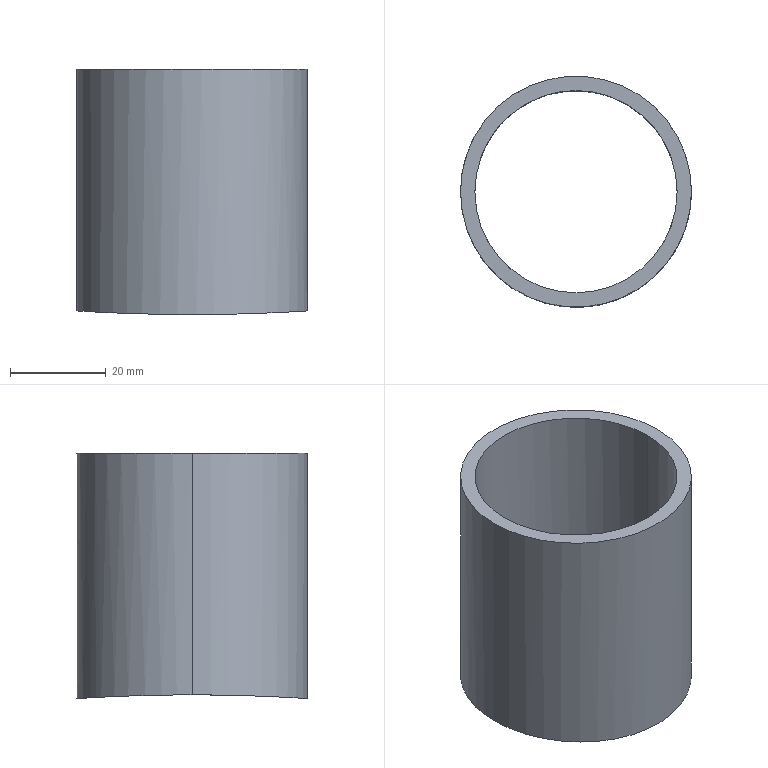Part | SolidWorks | features Extrusion 1, ICE 1 | 1 solid | 6 faces | box 48.3 x 48.3 x 51.269 mm | volume 21706 mm3 | cylinder 5 | plane 1 | commonest cylinder face diameters 42.3 x2 48.3 x2 759 x1
STEP:
#1=CARTESIAN_POINT('',(-21.15,0.,100.));
#2=VERTEX_POINT('',#1);
#3=CARTESIAN_POINT('',(21.15,0.,100.));
#4=VERTEX_POINT('',#3);
#5=CARTESIAN_POINT('',(0.,0.,100.));
#6=DIRECTION('',(0.,0.,1.));
#7=DIRECTION('',(1.,0.,0.));
#8=AXIS2_PLACEMENT_3D('',#5,#6,#7);
#9=CIRCLE('',#8,21.15);
#10=EDGE_CURVE('',#2,#4,#9,.T.);
#11=ORIENTED_EDGE('',*,*,#10,.T.);
#12=CARTESIAN_POINT('',(21.15,0.,49.5));
#13=VERTEX_POINT('',#12);
#14=CARTESIAN_POINT('',(21.15,0.,100.));
#15=DIRECTION('',(0.,0.,-1.));
#16=VECTOR('',#15,1000.);
#17=LINE('',#14,#16);
#18=EDGE_CURVE('',#4,#13,#17,.T.);
#19=ORIENTED_EDGE('',*,*,#18,.T.);
#20=CARTESIAN_POINT('',(-21.15,0.,49.5));
#21=VERTEX_POINT('',#20);
#22=CARTESIAN_POINT('',(-21.15,0.,49.5));
#23=CARTESIAN_POINT('',(-21.15,-1.398,49.5));
#24=CARTESIAN_POINT('',(-21.013,-2.772,49.492));
#25=CARTESIAN_POINT('',(-20.61,-4.8,49.47));
#26=CARTESIAN_POINT('',(-20.442,-5.47,49.461));
#27=CARTESIAN_POINT('',(-20.039,-6.799,49.44));
#28=CARTESIAN_POINT('',(-19.803,-7.46,49.427));
#29=CARTESIAN_POINT('',(-19.007,-9.381,49.386));
#30=CARTESIAN_POINT('',(-18.357,-10.595,49.354));
#31=CARTESIAN_POINT('',(-17.205,-12.32,49.3));
#32=CARTESIAN_POINT('',(-16.79,-12.88,49.282));
#33=CARTESIAN_POINT('',(-15.906,-13.958,49.244));
#34=CARTESIAN_POINT('',(-15.44,-14.47,49.224));
#35=CARTESIAN_POINT('',(-13.977,-15.933,49.167));
#36=CARTESIAN_POINT('',(-12.912,-16.809,49.128));
#37=CARTESIAN_POINT('',(-11.467,-17.775,49.084));
#38=CARTESIAN_POINT('',(-11.171,-17.962,49.075));
#39=CARTESIAN_POINT('',(-10.574,-18.32,49.058));
#40=CARTESIAN_POINT('',(-10.272,-18.491,49.049));
#41=CARTESIAN_POINT('',(-9.356,-18.981,49.025));
#42=CARTESIAN_POINT('',(-8.109,-19.57,48.995));
#43=CARTESIAN_POINT('',(-6.811,-20.035,48.971));
#44=CARTESIAN_POINT('',(-5.818,-20.337,48.955));
#45=CARTESIAN_POINT('',(-5.483,-20.43,48.95));
#46=CARTESIAN_POINT('',(-4.808,-20.599,48.941));
#47=CARTESIAN_POINT('',(-4.467,-20.676,48.936));
#48=CARTESIAN_POINT('',(-2.76,-21.015,48.918));
#49=CARTESIAN_POINT('',(-1.387,-21.15,48.91));
#50=CARTESIAN_POINT('',(0.6823,-21.15,48.91));
#51=CARTESIAN_POINT('',(1.374,-21.117,48.912));
#52=CARTESIAN_POINT('',(2.414,-21.015,48.918));
#53=CARTESIAN_POINT('',(2.762,-20.972,48.92));
#54=CARTESIAN_POINT('',(3.45,-20.87,48.926));
#55=CARTESIAN_POINT('',(3.791,-20.81,48.929));
#56=CARTESIAN_POINT('',(5.487,-20.473,48.947));
#57=CARTESIAN_POINT('',(6.805,-20.073,48.969));
#58=CARTESIAN_POINT('',(8.726,-19.278,49.01));
#59=CARTESIAN_POINT('',(9.36,-18.979,49.025));
#60=CARTESIAN_POINT('',(10.585,-18.324,49.058));
#61=CARTESIAN_POINT('',(11.178,-17.968,49.075));
#62=CARTESIAN_POINT('',(12.896,-16.82,49.128));
#63=CARTESIAN_POINT('',(13.965,-15.946,49.166));
#64=CARTESIAN_POINT('',(15.94,-13.971,49.244));
#65=CARTESIAN_POINT('',(16.816,-12.902,49.282));
#66=CARTESIAN_POINT('',(17.964,-11.184,49.336));
#67=CARTESIAN_POINT('',(18.32,-10.592,49.353));
#68=CARTESIAN_POINT('',(18.975,-9.368,49.385));
#69=CARTESIAN_POINT('',(19.275,-8.734,49.4));
#70=CARTESIAN_POINT('',(20.071,-6.812,49.441));
#71=CARTESIAN_POINT('',(20.471,-5.493,49.463));
#72=CARTESIAN_POINT('',(20.876,-3.46,49.485));
#73=CARTESIAN_POINT('',(20.979,-2.772,49.491));
#74=CARTESIAN_POINT('',(21.116,-1.383,49.498));
#75=CARTESIAN_POINT('',(21.15,-0.6902,49.5));
#76=CARTESIAN_POINT('',(21.15,0.,49.5));
#77=B_SPLINE_CURVE_WITH_KNOTS('',3,(#22,#23,#24,#25,#26,#27,#28,#29,#30,#31,#32,#33,#34,#35,#36,#37,#38,#39,#40,#41,#42,#43,#44,#45,#46,#47,#48,#49,#50,#51,#52,#53,#54,#55,#56,#57,#58,#59,#60,#61,#62,#63,#64,#65,#66,#67,#68,#69,#70,#71,#72,#73,#74,#75,#76),.UNSPECIFIED.,.F.,.F.,(4,2,2,2,2,2,2,2,2,2,1,2,2,2,2,2,2,2,2,2,2,2,2,2,2,2,2,4),(0.,0.004134,0.0062,0.008267,0.0124,0.01447,0.01653,0.02067,0.0217,0.02273,0.0248,0.02687,0.0279,0.02894,0.03307,0.03514,0.03617,0.0372,0.04134,0.0434,0.04547,0.0496,0.05374,0.0558,0.05787,0.062,0.06407,0.06614),.UNSPECIFIED.);
#78=EDGE_CURVE('',#21,#13,#77,.T.);
#79=ORIENTED_EDGE('',*,*,#78,.F.);
#80=CARTESIAN_POINT('',(-21.15,0.,100.));
#81=DIRECTION('',(0.,0.,-1.));
#82=VECTOR('',#81,1000.);
#83=LINE('',#80,#82);
#84=EDGE_CURVE('',#2,#21,#83,.T.);
#85=ORIENTED_EDGE('',*,*,#84,.F.);
#86=EDGE_LOOP('',(#11,#19,#79,#85));
#87=FACE_OUTER_BOUND('',#86,.T.);
#88=CARTESIAN_POINT('',(0.,0.,100.));
#89=DIRECTION('',(0.,0.,-1.));
#90=DIRECTION('',(-1.,0.,0.));
#91=AXIS2_PLACEMENT_3D('',#88,#89,#90);
#92=CYLINDRICAL_SURFACE('',#91,21.15);
#93=ADVANCED_FACE('',(#87),#92,.F.);
#94=CARTESIAN_POINT('',(24.15,0.,100.));
#95=VERTEX_POINT('',#94);
#96=CARTESIAN_POINT('',(-24.15,0.,100.));
#97=VERTEX_POINT('',#96);
#98=CARTESIAN_POINT('',(0.,0.,100.));
#99=DIRECTION('',(0.,0.,1.));
#100=DIRECTION('',(1.,0.,0.));
#101=AXIS2_PLACEMENT_3D('',#98,#99,#100);
#102=CIRCLE('',#101,24.15);
#103=EDGE_CURVE('',#95,#97,#102,.T.);
#104=ORIENTED_EDGE('',*,*,#103,.F.);
#105=CARTESIAN_POINT('',(24.15,0.,49.5));
#106=VERTEX_POINT('',#105);
#107=CARTESIAN_POINT('',(24.15,0.,100.));
#108=DIRECTION('',(0.,0.,-1.));
#109=VECTOR('',#108,1000.);
#110=LINE('',#107,#109);
#111=EDGE_CURVE('',#95,#106,#110,.T.);
#112=ORIENTED_EDGE('',*,*,#111,.T.);
#113=CARTESIAN_POINT('',(-24.15,0.,49.5));
#114=VERTEX_POINT('',#113);
#115=CARTESIAN_POINT('',(24.15,0.,49.5));
#116=CARTESIAN_POINT('',(24.15,1.576,49.5));
#117=CARTESIAN_POINT('',(23.997,3.143,49.49));
#118=CARTESIAN_POINT('',(23.611,5.089,49.466));
#119=CARTESIAN_POINT('',(23.524,5.479,49.461));
#120=CARTESIAN_POINT('',(23.331,6.25,49.449));
#121=CARTESIAN_POINT('',(23.225,6.633,49.442));
#122=CARTESIAN_POINT('',(22.88,7.767,49.421));
#123=CARTESIAN_POINT('',(22.35,9.25,49.389));
#124=CARTESIAN_POINT('',(21.678,10.674,49.351));
#125=CARTESIAN_POINT('',(21.12,11.719,49.319));
#126=CARTESIAN_POINT('',(20.925,12.063,49.308));
#127=CARTESIAN_POINT('',(20.517,12.745,49.286));
#128=CARTESIAN_POINT('',(20.303,13.082,49.275));
#129=CARTESIAN_POINT('',(19.2,14.734,49.216));
#130=CARTESIAN_POINT('',(18.201,15.951,49.166));
#131=CARTESIAN_POINT('',(16.532,17.622,49.091));
#132=CARTESIAN_POINT('',(15.948,18.153,49.066));
#133=CARTESIAN_POINT('',(15.027,18.91,49.029));
#134=CARTESIAN_POINT('',(14.712,19.156,49.016));
#135=CARTESIAN_POINT('',(14.074,19.629,48.992));
#136=CARTESIAN_POINT('',(13.751,19.857,48.98));
#137=CARTESIAN_POINT('',(12.11,20.954,48.922));
#138=CARTESIAN_POINT('',(10.724,21.696,48.88));
#139=CARTESIAN_POINT('',(8.899,22.454,48.835));
#140=CARTESIAN_POINT('',(8.529,22.597,48.827));
#141=CARTESIAN_POINT('',(7.78,22.866,48.811));
#142=CARTESIAN_POINT('',(7.401,22.992,48.803));
#143=CARTESIAN_POINT('',(6.262,23.338,48.782));
#144=CARTESIAN_POINT('',(5.496,23.529,48.77));
#145=CARTESIAN_POINT('',(3.181,23.991,48.741));
#146=CARTESIAN_POINT('',(1.613,24.149,48.731));
#147=CARTESIAN_POINT('',(-0.7771,24.151,48.731));
#148=CARTESIAN_POINT('',(-1.571,24.112,48.733));
#149=CARTESIAN_POINT('',(-3.141,23.958,48.743));
#150=CARTESIAN_POINT('',(-3.92,23.843,48.75));
#151=CARTESIAN_POINT('',(-5.463,23.537,48.769));
#152=CARTESIAN_POINT('',(-6.228,23.347,48.781));
#153=CARTESIAN_POINT('',(-7.744,22.888,48.809));
#154=CARTESIAN_POINT('',(-8.498,22.619,48.825));
#155=CARTESIAN_POINT('',(-10.694,21.711,48.879));
#156=CARTESIAN_POINT('',(-12.082,20.97,48.921));
#157=CARTESIAN_POINT('',(-14.05,19.658,48.991));
#158=CARTESIAN_POINT('',(-14.688,19.186,49.015));
#159=CARTESIAN_POINT('',(-15.921,18.177,49.065));
#160=CARTESIAN_POINT('',(-16.507,17.645,49.09));
#161=CARTESIAN_POINT('',(-18.179,15.975,49.165));
#162=CARTESIAN_POINT('',(-19.179,14.761,49.215));
#163=CARTESIAN_POINT('',(-20.504,12.785,49.285));
#164=CARTESIAN_POINT('',(-20.916,12.099,49.308));
#165=CARTESIAN_POINT('',(-21.662,10.704,49.35));
#166=CARTESIAN_POINT('',(-22.,9.993,49.369));
#167=CARTESIAN_POINT('',(-22.603,8.54,49.405));
#168=CARTESIAN_POINT('',(-22.869,7.8,49.421));
#169=CARTESIAN_POINT('',(-23.33,6.29,49.449));
#170=CARTESIAN_POINT('',(-23.525,5.517,49.461));
#171=CARTESIAN_POINT('',(-23.993,3.174,49.49));
#172=CARTESIAN_POINT('',(-24.15,1.596,49.5));
#173=CARTESIAN_POINT('',(-24.15,0.,49.5));
#174=B_SPLINE_CURVE_WITH_KNOTS('',3,(#115,#116,#117,#118,#119,#120,#121,#122,#123,#124,#125,#126,#127,#128,#129,#130,#131,#132,#133,#134,#135,#136,#137,#138,#139,#140,#141,#142,#143,#144,#145,#146,#147,#148,#149,#150,#151,#152,#153,#154,#155,#156,#157,#158,#159,#160,#161,#162,#163,#164,#165,#166,#167,#168,#169,#170,#171,#172,#173),.UNSPECIFIED.,.F.,.F.,(4,2,2,2,1,2,2,2,2,2,2,2,2,2,2,2,2,2,2,2,2,2,2,2,2,2,2,2,2,4),(0.07552,0.08024,0.08142,0.0826,0.08496,0.08732,0.0885,0.08968,0.0944,0.09676,0.09794,0.09912,0.1038,0.105,0.1062,0.1086,0.1133,0.1156,0.118,0.1204,0.1227,0.1274,0.1298,0.1322,0.1369,0.1392,0.1416,0.144,0.1463,0.151),.UNSPECIFIED.);
#175=EDGE_CURVE('',#106,#114,#174,.T.);
#176=ORIENTED_EDGE('',*,*,#175,.T.);
#177=CARTESIAN_POINT('',(-24.15,0.,100.));
#178=DIRECTION('',(0.,0.,-1.));
#179=VECTOR('',#178,1000.);
#180=LINE('',#177,#179);
#181=EDGE_CURVE('',#97,#114,#180,.T.);
#182=ORIENTED_EDGE('',*,*,#181,.F.);
#183=EDGE_LOOP('',(#104,#112,#176,#182));
#184=FACE_OUTER_BOUND('',#183,.T.);
#185=CARTESIAN_POINT('',(0.,0.,100.));
#186=DIRECTION('',(0.,0.,-1.));
#187=DIRECTION('',(-1.,0.,0.));
#188=AXIS2_PLACEMENT_3D('',#185,#186,#187);
#189=CYLINDRICAL_SURFACE('',#188,24.15);
#190=ADVANCED_FACE('',(#184),#189,.T.);
#191=CARTESIAN_POINT('',(0.,0.,100.));
#192=DIRECTION('',(0.,0.,1.));
#193=DIRECTION('',(1.,0.,0.));
#194=AXIS2_PLACEMENT_3D('',#191,#192,#193);
#195=CIRCLE('',#194,24.15);
#196=EDGE_CURVE('',#97,#95,#195,.T.);
#197=ORIENTED_EDGE('',*,*,#196,.T.);
#198=ORIENTED_EDGE('',*,*,#103,.T.);
#199=EDGE_LOOP('',(#197,#198));
#200=FACE_OUTER_BOUND('',#199,.T.);
#201=ORIENTED_EDGE('',*,*,#10,.F.);
#202=CARTESIAN_POINT('',(0.,0.,100.));
#203=DIRECTION('',(0.,0.,1.));
#204=DIRECTION('',(1.,0.,0.));
#205=AXIS2_PLACEMENT_3D('',#202,#203,#204);
#206=CIRCLE('',#205,21.15);
#207=EDGE_CURVE('',#4,#2,#206,.T.);
#208=ORIENTED_EDGE('',*,*,#207,.F.);
#209=EDGE_LOOP('',(#201,#208));
#210=FACE_BOUND('',#209,.T.);
#211=CARTESIAN_POINT('',(0.,0.,100.));
#212=DIRECTION('',(0.,0.,1.));
#213=DIRECTION('',(1.,0.,0.));
#214=AXIS2_PLACEMENT_3D('',#211,#212,#213);
#215=PLANE('',#214);
#216=ADVANCED_FACE('',(#200,#210),#215,.T.);
#217=ORIENTED_EDGE('',*,*,#111,.F.);
#218=ORIENTED_EDGE('',*,*,#196,.F.);
#219=ORIENTED_EDGE('',*,*,#181,.T.);
#220=CARTESIAN_POINT('',(-24.15,0.,49.5));
#221=CARTESIAN_POINT('',(-24.15,-1.596,49.5));
#222=CARTESIAN_POINT('',(-23.993,-3.165,49.49));
#223=CARTESIAN_POINT('',(-23.533,-5.481,49.461));
#224=CARTESIAN_POINT('',(-23.342,-6.246,49.449));
#225=CARTESIAN_POINT('',(-22.882,-7.764,49.421));
#226=CARTESIAN_POINT('',(-22.612,-8.518,49.405));
#227=CARTESIAN_POINT('',(-21.702,-10.711,49.352));
#228=CARTESIAN_POINT('',(-20.96,-12.099,49.309));
#229=CARTESIAN_POINT('',(-19.865,-13.739,49.251));
#230=CARTESIAN_POINT('',(-19.637,-14.063,49.239));
#231=CARTESIAN_POINT('',(-19.165,-14.7,49.215));
#232=CARTESIAN_POINT('',(-18.919,-15.015,49.203));
#233=CARTESIAN_POINT('',(-18.162,-15.937,49.166));
#234=CARTESIAN_POINT('',(-17.63,-16.523,49.141));
#235=CARTESIAN_POINT('',(-15.959,-18.193,49.065));
#236=CARTESIAN_POINT('',(-14.744,-19.193,49.015));
#237=CARTESIAN_POINT('',(-13.094,-20.296,48.957));
#238=CARTESIAN_POINT('',(-12.756,-20.51,48.945));
#239=CARTESIAN_POINT('',(-12.074,-20.919,48.923));
#240=CARTESIAN_POINT('',(-11.729,-21.114,48.912));
#241=CARTESIAN_POINT('',(-10.684,-21.673,48.881));
#242=CARTESIAN_POINT('',(-9.26,-22.346,48.842));
#243=CARTESIAN_POINT('',(-7.777,-22.877,48.81));
#244=CARTESIAN_POINT('',(-6.643,-23.222,48.789));
#245=CARTESIAN_POINT('',(-6.261,-23.328,48.782));
#246=CARTESIAN_POINT('',(-5.49,-23.521,48.77));
#247=CARTESIAN_POINT('',(-5.1,-23.609,48.765));
#248=CARTESIAN_POINT('',(-3.152,-23.996,48.741));
#249=CARTESIAN_POINT('',(-1.584,-24.149,48.731));
#250=CARTESIAN_POINT('',(0.7792,-24.15,48.731));
#251=CARTESIAN_POINT('',(1.569,-24.112,48.733));
#252=CARTESIAN_POINT('',(2.757,-23.995,48.741));
#253=CARTESIAN_POINT('',(3.154,-23.946,48.744));
#254=CARTESIAN_POINT('',(3.939,-23.83,48.751));
#255=CARTESIAN_POINT('',(4.329,-23.762,48.755));
#256=CARTESIAN_POINT('',(6.265,-23.377,48.779));
#257=CARTESIAN_POINT('',(7.771,-22.92,48.808));
#258=CARTESIAN_POINT('',(9.964,-22.013,48.861));
#259=CARTESIAN_POINT('',(10.688,-21.671,48.881));
#260=CARTESIAN_POINT('',(12.087,-20.923,48.923));
#261=CARTESIAN_POINT('',(12.763,-20.517,48.945));
#262=CARTESIAN_POINT('',(14.726,-19.205,49.015));
#263=CARTESIAN_POINT('',(15.945,-18.207,49.065));
#264=CARTESIAN_POINT('',(18.201,-15.953,49.166));
#265=CARTESIAN_POINT('',(19.201,-14.732,49.216));
#266=CARTESIAN_POINT('',(20.512,-12.77,49.286));
#267=CARTESIAN_POINT('',(20.918,-12.094,49.308));
#268=CARTESIAN_POINT('',(21.666,-10.697,49.35));
#269=CARTESIAN_POINT('',(22.009,-9.973,49.37));
#270=CARTESIAN_POINT('',(22.918,-7.778,49.423));
#271=CARTESIAN_POINT('',(23.374,-6.273,49.451));
#272=CARTESIAN_POINT('',(23.838,-3.951,49.48));
#273=CARTESIAN_POINT('',(23.955,-3.165,49.488));
#274=CARTESIAN_POINT('',(24.112,-1.579,49.498));
#275=CARTESIAN_POINT('',(24.15,-0.7882,49.5));
#276=CARTESIAN_POINT('',(24.15,0.,49.5));
#277=B_SPLINE_CURVE_WITH_KNOTS('',3,(#220,#221,#222,#223,#224,#225,#226,#227,#228,#229,#230,#231,#232,#233,#234,#235,#236,#237,#238,#239,#240,#241,#242,#243,#244,#245,#246,#247,#248,#249,#250,#251,#252,#253,#254,#255,#256,#257,#258,#259,#260,#261,#262,#263,#264,#265,#266,#267,#268,#269,#270,#271,#272,#273,#274,#275,#276),.UNSPECIFIED.,.F.,.F.,(4,2,2,2,2,2,2,2,2,2,2,1,2,2,2,2,2,2,2,2,2,2,2,2,2,2,2,2,4),(0.,0.00472,0.00708,0.00944,0.01416,0.01534,0.01652,0.01888,0.0236,0.02478,0.02596,0.02832,0.03068,0.03186,0.03304,0.03776,0.04012,0.0413,0.04248,0.0472,0.04956,0.05192,0.05664,0.06136,0.06372,0.06608,0.0708,0.07316,0.07552),.UNSPECIFIED.);
#278=EDGE_CURVE('',#114,#106,#277,.T.);
#279=ORIENTED_EDGE('',*,*,#278,.T.);
#280=EDGE_LOOP('',(#217,#218,#219,#279));
#281=FACE_OUTER_BOUND('',#280,.T.);
#282=CARTESIAN_POINT('',(0.,0.,100.));
#283=DIRECTION('',(0.,0.,-1.));
#284=DIRECTION('',(-1.,0.,0.));
#285=AXIS2_PLACEMENT_3D('',#282,#283,#284);
#286=CYLINDRICAL_SURFACE('',#285,24.15);
#287=ADVANCED_FACE('',(#281),#286,.T.);
#288=ORIENTED_EDGE('',*,*,#18,.F.);
#289=ORIENTED_EDGE('',*,*,#207,.T.);
#290=ORIENTED_EDGE('',*,*,#84,.T.);
#291=CARTESIAN_POINT('',(21.15,0.,49.5));
#292=CARTESIAN_POINT('',(21.15,1.38,49.5));
#293=CARTESIAN_POINT('',(21.016,2.752,49.492));
#294=CARTESIAN_POINT('',(20.61,4.797,49.47));
#295=CARTESIAN_POINT('',(20.44,5.477,49.461));
#296=CARTESIAN_POINT('',(20.038,6.802,49.44));
#297=CARTESIAN_POINT('',(19.573,8.101,49.415));
#298=CARTESIAN_POINT('',(18.985,9.348,49.385));
#299=CARTESIAN_POINT('',(18.496,10.263,49.361));
#300=CARTESIAN_POINT('',(18.326,10.564,49.353));
#301=CARTESIAN_POINT('',(17.969,11.161,49.336));
#302=CARTESIAN_POINT('',(17.782,11.457,49.327));
#303=CARTESIAN_POINT('',(16.815,12.904,49.282));
#304=CARTESIAN_POINT('',(15.94,13.969,49.244));
#305=CARTESIAN_POINT('',(14.479,15.433,49.186));
#306=CARTESIAN_POINT('',(13.967,15.898,49.167));
#307=CARTESIAN_POINT('',(13.16,16.561,49.139));
#308=CARTESIAN_POINT('',(12.884,16.776,49.129));
#309=CARTESIAN_POINT('',(12.326,17.191,49.111));
#310=CARTESIAN_POINT('',(12.043,17.39,49.101));
#311=CARTESIAN_POINT('',(10.606,18.351,49.057));
#312=CARTESIAN_POINT('',(9.391,19.001,49.024));
#313=CARTESIAN_POINT('',(7.473,19.798,48.983));
#314=CARTESIAN_POINT('',(6.814,20.034,48.971));
#315=CARTESIAN_POINT('',(5.484,20.439,48.949));
#316=CARTESIAN_POINT('',(4.813,20.607,48.94));
#317=CARTESIAN_POINT('',(2.786,21.011,48.918));
#318=CARTESIAN_POINT('',(1.413,21.149,48.91));
#319=CARTESIAN_POINT('',(-0.6803,21.151,48.91));
#320=CARTESIAN_POINT('',(-1.376,21.117,48.912));
#321=CARTESIAN_POINT('',(-2.751,20.982,48.92));
#322=CARTESIAN_POINT('',(-3.433,20.881,48.925));
#323=CARTESIAN_POINT('',(-4.784,20.613,48.94));
#324=CARTESIAN_POINT('',(-5.454,20.446,48.949));
#325=CARTESIAN_POINT('',(-6.782,20.045,48.97));
#326=CARTESIAN_POINT('',(-7.442,19.81,48.983));
#327=CARTESIAN_POINT('',(-9.366,19.014,49.024));
#328=CARTESIAN_POINT('',(-10.581,18.365,49.056));
#329=CARTESIAN_POINT('',(-12.304,17.216,49.109));
#330=CARTESIAN_POINT('',(-12.863,16.803,49.128));
#331=CARTESIAN_POINT('',(-13.943,15.919,49.166));
#332=CARTESIAN_POINT('',(-14.456,15.453,49.186));
#333=CARTESIAN_POINT('',(-15.921,13.991,49.243));
#334=CARTESIAN_POINT('',(-16.797,12.927,49.282));
#335=CARTESIAN_POINT('',(-17.957,11.197,49.335));
#336=CARTESIAN_POINT('',(-18.318,10.596,49.353));
#337=CARTESIAN_POINT('',(-18.972,9.374,49.385));
#338=CARTESIAN_POINT('',(-19.267,8.751,49.4));
#339=CARTESIAN_POINT('',(-19.795,7.479,49.427));
#340=CARTESIAN_POINT('',(-20.029,6.831,49.439));
#341=CARTESIAN_POINT('',(-20.432,5.508,49.461));
#342=CARTESIAN_POINT('',(-20.602,4.832,49.47));
#343=CARTESIAN_POINT('',(-21.013,2.78,49.492));
#344=CARTESIAN_POINT('',(-21.15,1.397,49.5));
#345=CARTESIAN_POINT('',(-21.15,0.,49.5));
#346=B_SPLINE_CURVE_WITH_KNOTS('',3,(#291,#292,#293,#294,#295,#296,#297,#298,#299,#300,#301,#302,#303,#304,#305,#306,#307,#308,#309,#310,#311,#312,#313,#314,#315,#316,#317,#318,#319,#320,#321,#322,#323,#324,#325,#326,#327,#328,#329,#330,#331,#332,#333,#334,#335,#336,#337,#338,#339,#340,#341,#342,#343,#344,#345),.UNSPECIFIED.,.F.,.F.,(4,2,2,1,2,2,2,2,2,2,2,2,2,2,2,2,2,2,2,2,2,2,2,2,2,2,2,4),(0.06614,0.07027,0.07234,0.0744,0.07647,0.0775,0.07854,0.08267,0.08473,0.08577,0.0868,0.09093,0.093,0.09507,0.0992,0.1013,0.1033,0.1054,0.1075,0.1116,0.1137,0.1157,0.1199,0.1219,0.124,0.1261,0.1281,0.1323),.UNSPECIFIED.);
#347=EDGE_CURVE('',#13,#21,#346,.T.);
#348=ORIENTED_EDGE('',*,*,#347,.F.);
#349=EDGE_LOOP('',(#288,#289,#290,#348));
#350=FACE_OUTER_BOUND('',#349,.T.);
#351=CARTESIAN_POINT('',(0.,0.,100.));
#352=DIRECTION('',(0.,0.,-1.));
#353=DIRECTION('',(-1.,0.,0.));
#354=AXIS2_PLACEMENT_3D('',#351,#352,#353);
#355=CYLINDRICAL_SURFACE('',#354,21.15);
#356=ADVANCED_FACE('',(#350),#355,.F.);
#357=ORIENTED_EDGE('',*,*,#78,.T.);
#358=ORIENTED_EDGE('',*,*,#347,.T.);
#359=EDGE_LOOP('',(#357,#358));
#360=FACE_BOUND('',#359,.T.);
#361=ORIENTED_EDGE('',*,*,#278,.F.);
#362=ORIENTED_EDGE('',*,*,#175,.F.);
#363=EDGE_LOOP('',(#361,#362));
#364=FACE_OUTER_BOUND('',#363,.T.);
#365=CARTESIAN_POINT('',(-50.,0.,-330.));
#366=DIRECTION('',(1.,0.,0.));
#367=DIRECTION('',(0.,0.,-1.));
#368=AXIS2_PLACEMENT_3D('',#365,#366,#367);
#369=CYLINDRICAL_SURFACE('',#368,379.5);
#370=ADVANCED_FACE('',(#360,#364),#369,.F.);
#371=CLOSED_SHELL('',(#93,#190,#216,#287,#356,#370));
#372=MANIFOLD_SOLID_BREP('',#371);
#373=CARTESIAN_POINT('',(0.,0.,0.));
#374=DIRECTION('',(0.,0.,1.));
#375=DIRECTION('',(1.,0.,0.));
#376=AXIS2_PLACEMENT_3D('',#373,#374,#375);
#377=(LENGTH_UNIT()NAMED_UNIT(*)SI_UNIT(.MILLI.,.METRE.));
#378=UNCERTAINTY_MEASURE_WITH_UNIT(LENGTH_MEASURE(0.00001),#377,'','');
#379=(NAMED_UNIT(*)PLANE_ANGLE_UNIT()SI_UNIT($,.RADIAN.));
#380=(NAMED_UNIT(*)SI_UNIT($,.STERADIAN.)SOLID_ANGLE_UNIT());
#381=(GEOMETRIC_REPRESENTATION_CONTEXT(3)GLOBAL_UNCERTAINTY_ASSIGNED_CONTEXT((#378))GLOBAL_UNIT_ASSIGNED_CONTEXT((#377,#379,#380))REPRESENTATION_CONTEXT('',''));
#382=ADVANCED_BREP_SHAPE_REPRESENTATION('',(#372,#376),#381);